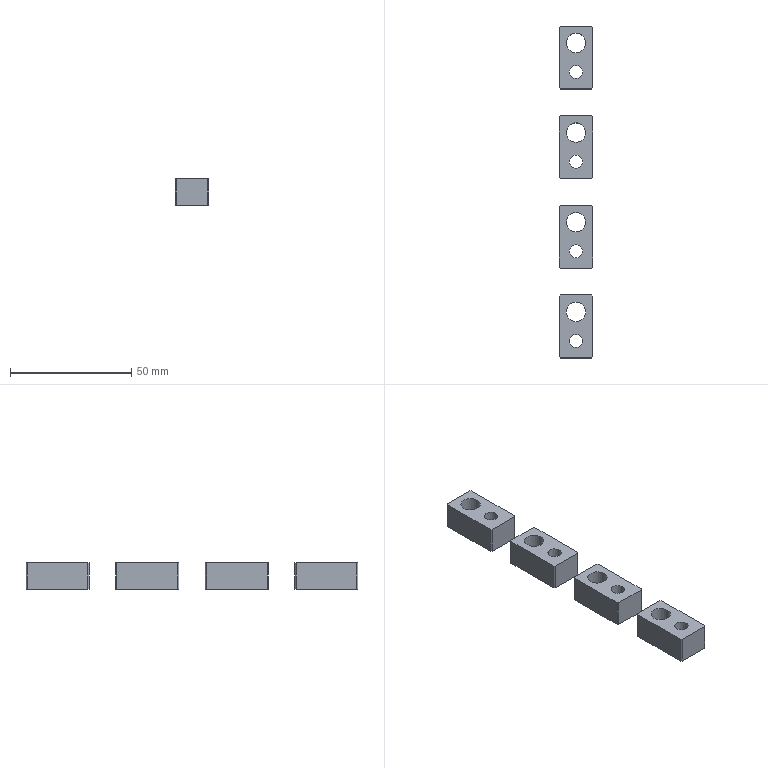Part | 4 solids | 56 faces | box 14 x 137 x 11 mm | volume 11860 mm3 | plane 44 | cylinder 12 | commonest cylinder face diameters 5.5 x4 8 x4 9 x4
STEP:
#1=CARTESIAN_POINT('',(-323.995,269.879,-17.));
#2=VERTEX_POINT('',#1);
#3=CARTESIAN_POINT('',(-321.245,269.879,-17.));
#4=DIRECTION('',(0.,0.,-1.));
#5=DIRECTION('',(-1.,0.,0.));
#6=AXIS2_PLACEMENT_3D('',#3,#4,#5);
#7=CIRCLE('',#6,2.75);
#8=EDGE_CURVE('',#2,#2,#7,.T.);
#9=ORIENTED_EDGE('',*,*,#8,.T.);
#10=EDGE_LOOP('',(#9));
#11=FACE_BOUND('',#10,.T.);
#12=CARTESIAN_POINT('',(-317.245,281.879,-17.));
#13=VERTEX_POINT('',#12);
#14=CARTESIAN_POINT('',(-321.245,281.879,-17.));
#15=DIRECTION('',(0.,0.,1.));
#16=DIRECTION('',(1.,0.,0.));
#17=AXIS2_PLACEMENT_3D('',#14,#15,#16);
#18=CIRCLE('',#17,4.);
#19=EDGE_CURVE('',#13,#13,#18,.T.);
#20=ORIENTED_EDGE('',*,*,#19,.F.);
#21=EDGE_LOOP('',(#20));
#22=FACE_BOUND('',#21,.T.);
#23=CARTESIAN_POINT('',(-328.245,288.379,-17.));
#24=VERTEX_POINT('',#23);
#25=CARTESIAN_POINT('',(-327.745,288.879,-17.));
#26=VERTEX_POINT('',#25);
#27=CARTESIAN_POINT('',(-333.995,282.629,-17.));
#28=DIRECTION('',(0.7071,0.7071,0.));
#29=VECTOR('',#28,1000.);
#30=LINE('',#27,#29);
#31=EDGE_CURVE('',#24,#26,#30,.T.);
#32=ORIENTED_EDGE('',*,*,#31,.F.);
#33=CARTESIAN_POINT('',(-328.245,263.379,-17.));
#34=VERTEX_POINT('',#33);
#35=CARTESIAN_POINT('',(-328.245,269.879,-17.));
#36=DIRECTION('',(0.,-1.,0.));
#37=VECTOR('',#36,1000.);
#38=LINE('',#35,#37);
#39=EDGE_CURVE('',#24,#34,#38,.T.);
#40=ORIENTED_EDGE('',*,*,#39,.T.);
#41=CARTESIAN_POINT('',(-327.745,262.879,-17.));
#42=VERTEX_POINT('',#41);
#43=CARTESIAN_POINT('',(-327.995,263.129,-17.));
#44=DIRECTION('',(-0.7071,0.7071,0.));
#45=VECTOR('',#44,1000.);
#46=LINE('',#43,#45);
#47=EDGE_CURVE('',#42,#34,#46,.T.);
#48=ORIENTED_EDGE('',*,*,#47,.F.);
#49=CARTESIAN_POINT('',(-314.745,262.879,-17.));
#50=VERTEX_POINT('',#49);
#51=CARTESIAN_POINT('',(-321.245,262.879,-17.));
#52=DIRECTION('',(1.,0.,0.));
#53=VECTOR('',#52,1000.);
#54=LINE('',#51,#53);
#55=EDGE_CURVE('',#42,#50,#54,.T.);
#56=ORIENTED_EDGE('',*,*,#55,.T.);
#57=CARTESIAN_POINT('',(-314.245,263.379,-17.));
#58=VERTEX_POINT('',#57);
#59=CARTESIAN_POINT('',(-314.495,263.129,-17.));
#60=DIRECTION('',(-0.7071,-0.7071,0.));
#61=VECTOR('',#60,1000.);
#62=LINE('',#59,#61);
#63=EDGE_CURVE('',#58,#50,#62,.T.);
#64=ORIENTED_EDGE('',*,*,#63,.F.);
#65=CARTESIAN_POINT('',(-314.245,288.379,-17.));
#66=VERTEX_POINT('',#65);
#67=CARTESIAN_POINT('',(-314.245,269.879,-17.));
#68=DIRECTION('',(0.,1.,0.));
#69=VECTOR('',#68,1000.);
#70=LINE('',#67,#69);
#71=EDGE_CURVE('',#58,#66,#70,.T.);
#72=ORIENTED_EDGE('',*,*,#71,.T.);
#73=CARTESIAN_POINT('',(-314.745,288.879,-17.));
#74=VERTEX_POINT('',#73);
#75=CARTESIAN_POINT('',(-308.495,282.629,-17.));
#76=DIRECTION('',(0.7071,-0.7071,0.));
#77=VECTOR('',#76,1000.);
#78=LINE('',#75,#77);
#79=EDGE_CURVE('',#74,#66,#78,.T.);
#80=ORIENTED_EDGE('',*,*,#79,.F.);
#81=CARTESIAN_POINT('',(-321.245,288.879,-17.));
#82=DIRECTION('',(-1.,0.,0.));
#83=VECTOR('',#82,1000.);
#84=LINE('',#81,#83);
#85=EDGE_CURVE('',#74,#26,#84,.T.);
#86=ORIENTED_EDGE('',*,*,#85,.T.);
#87=EDGE_LOOP('',(#32,#40,#48,#56,#64,#72,#80,#86));
#88=FACE_BOUND('',#87,.T.);
#89=CARTESIAN_POINT('',(-321.245,269.879,-17.));
#90=DIRECTION('',(0.,0.,1.));
#91=DIRECTION('',(-1.,0.,0.));
#92=AXIS2_PLACEMENT_3D('',#89,#90,#91);
#93=PLANE('',#92);
#94=ADVANCED_FACE('',(#11,#22,#88),#93,.T.);
#95=ORIENTED_EDGE('',*,*,#55,.F.);
#96=CARTESIAN_POINT('',(-327.745,262.879,-28.));
#97=VERTEX_POINT('',#96);
#98=CARTESIAN_POINT('',(-327.745,262.879,-16.));
#99=DIRECTION('',(0.,0.,-1.));
#100=VECTOR('',#99,1000.);
#101=LINE('',#98,#100);
#102=EDGE_CURVE('',#42,#97,#101,.T.);
#103=ORIENTED_EDGE('',*,*,#102,.T.);
#104=CARTESIAN_POINT('',(-314.745,262.879,-28.));
#105=VERTEX_POINT('',#104);
#106=CARTESIAN_POINT('',(-321.245,262.879,-28.));
#107=DIRECTION('',(-1.,0.,0.));
#108=VECTOR('',#107,1000.);
#109=LINE('',#106,#108);
#110=EDGE_CURVE('',#105,#97,#109,.T.);
#111=ORIENTED_EDGE('',*,*,#110,.F.);
#112=CARTESIAN_POINT('',(-314.745,262.879,-16.));
#113=DIRECTION('',(0.,0.,1.));
#114=VECTOR('',#113,1000.);
#115=LINE('',#112,#114);
#116=EDGE_CURVE('',#105,#50,#115,.T.);
#117=ORIENTED_EDGE('',*,*,#116,.T.);
#118=EDGE_LOOP('',(#95,#103,#111,#117));
#119=FACE_BOUND('',#118,.T.);
#120=CARTESIAN_POINT('',(-321.245,262.879,-16.));
#121=DIRECTION('',(0.,-1.,0.));
#122=DIRECTION('',(0.,0.,1.));
#123=AXIS2_PLACEMENT_3D('',#120,#121,#122);
#124=PLANE('',#123);
#125=ADVANCED_FACE('',(#119),#124,.T.);
#126=CARTESIAN_POINT('',(-314.245,263.379,-28.));
#127=VERTEX_POINT('',#126);
#128=CARTESIAN_POINT('',(-314.245,263.379,-16.));
#129=DIRECTION('',(0.,0.,-1.));
#130=VECTOR('',#129,1000.);
#131=LINE('',#128,#130);
#132=EDGE_CURVE('',#58,#127,#131,.T.);
#133=ORIENTED_EDGE('',*,*,#132,.F.);
#134=ORIENTED_EDGE('',*,*,#63,.T.);
#135=ORIENTED_EDGE('',*,*,#116,.F.);
#136=CARTESIAN_POINT('',(-314.495,263.129,-28.));
#137=DIRECTION('',(0.7071,0.7071,0.));
#138=VECTOR('',#137,1000.);
#139=LINE('',#136,#138);
#140=EDGE_CURVE('',#105,#127,#139,.T.);
#141=ORIENTED_EDGE('',*,*,#140,.T.);
#142=EDGE_LOOP('',(#133,#134,#135,#141));
#143=FACE_BOUND('',#142,.T.);
#144=CARTESIAN_POINT('',(-314.745,262.879,-16.));
#145=DIRECTION('',(-0.7071,0.7071,0.));
#146=DIRECTION('',(0.,0.,1.));
#147=AXIS2_PLACEMENT_3D('',#144,#145,#146);
#148=PLANE('',#147);
#149=ADVANCED_FACE('',(#143),#148,.F.);
#150=ORIENTED_EDGE('',*,*,#71,.F.);
#151=ORIENTED_EDGE('',*,*,#132,.T.);
#152=CARTESIAN_POINT('',(-314.245,288.379,-28.));
#153=VERTEX_POINT('',#152);
#154=CARTESIAN_POINT('',(-314.245,269.879,-28.));
#155=DIRECTION('',(0.,-1.,0.));
#156=VECTOR('',#155,1000.);
#157=LINE('',#154,#156);
#158=EDGE_CURVE('',#153,#127,#157,.T.);
#159=ORIENTED_EDGE('',*,*,#158,.F.);
#160=CARTESIAN_POINT('',(-314.245,288.379,-16.));
#161=DIRECTION('',(0.,0.,1.));
#162=VECTOR('',#161,1000.);
#163=LINE('',#160,#162);
#164=EDGE_CURVE('',#153,#66,#163,.T.);
#165=ORIENTED_EDGE('',*,*,#164,.T.);
#166=EDGE_LOOP('',(#150,#151,#159,#165));
#167=FACE_BOUND('',#166,.T.);
#168=CARTESIAN_POINT('',(-314.245,269.879,-16.));
#169=DIRECTION('',(1.,0.,0.));
#170=DIRECTION('',(0.,0.,1.));
#171=AXIS2_PLACEMENT_3D('',#168,#169,#170);
#172=PLANE('',#171);
#173=ADVANCED_FACE('',(#167),#172,.T.);
#174=CARTESIAN_POINT('',(-314.745,288.879,-28.));
#175=VERTEX_POINT('',#174);
#176=CARTESIAN_POINT('',(-314.745,288.879,-16.));
#177=DIRECTION('',(0.,0.,-1.));
#178=VECTOR('',#177,1000.);
#179=LINE('',#176,#178);
#180=EDGE_CURVE('',#74,#175,#179,.T.);
#181=ORIENTED_EDGE('',*,*,#180,.F.);
#182=ORIENTED_EDGE('',*,*,#79,.T.);
#183=ORIENTED_EDGE('',*,*,#164,.F.);
#184=CARTESIAN_POINT('',(-308.495,282.629,-28.));
#185=DIRECTION('',(-0.7071,0.7071,0.));
#186=VECTOR('',#185,1000.);
#187=LINE('',#184,#186);
#188=EDGE_CURVE('',#153,#175,#187,.T.);
#189=ORIENTED_EDGE('',*,*,#188,.T.);
#190=EDGE_LOOP('',(#181,#182,#183,#189));
#191=FACE_BOUND('',#190,.T.);
#192=CARTESIAN_POINT('',(-314.245,288.379,-16.));
#193=DIRECTION('',(-0.7071,-0.7071,0.));
#194=DIRECTION('',(0.,0.,1.));
#195=AXIS2_PLACEMENT_3D('',#192,#193,#194);
#196=PLANE('',#195);
#197=ADVANCED_FACE('',(#191),#196,.F.);
#198=ORIENTED_EDGE('',*,*,#85,.F.);
#199=ORIENTED_EDGE('',*,*,#180,.T.);
#200=CARTESIAN_POINT('',(-327.745,288.879,-28.));
#201=VERTEX_POINT('',#200);
#202=CARTESIAN_POINT('',(-321.245,288.879,-28.));
#203=DIRECTION('',(1.,0.,0.));
#204=VECTOR('',#203,1000.);
#205=LINE('',#202,#204);
#206=EDGE_CURVE('',#201,#175,#205,.T.);
#207=ORIENTED_EDGE('',*,*,#206,.F.);
#208=CARTESIAN_POINT('',(-327.745,288.879,-16.));
#209=DIRECTION('',(0.,0.,1.));
#210=VECTOR('',#209,1000.);
#211=LINE('',#208,#210);
#212=EDGE_CURVE('',#201,#26,#211,.T.);
#213=ORIENTED_EDGE('',*,*,#212,.T.);
#214=EDGE_LOOP('',(#198,#199,#207,#213));
#215=FACE_BOUND('',#214,.T.);
#216=CARTESIAN_POINT('',(-321.245,288.879,-16.));
#217=DIRECTION('',(0.,1.,0.));
#218=DIRECTION('',(0.,0.,-1.));
#219=AXIS2_PLACEMENT_3D('',#216,#217,#218);
#220=PLANE('',#219);
#221=ADVANCED_FACE('',(#215),#220,.T.);
#222=CARTESIAN_POINT('',(-328.245,288.379,-28.));
#223=VERTEX_POINT('',#222);
#224=CARTESIAN_POINT('',(-328.245,288.379,-16.));
#225=DIRECTION('',(0.,0.,-1.));
#226=VECTOR('',#225,1000.);
#227=LINE('',#224,#226);
#228=EDGE_CURVE('',#24,#223,#227,.T.);
#229=ORIENTED_EDGE('',*,*,#228,.F.);
#230=ORIENTED_EDGE('',*,*,#31,.T.);
#231=ORIENTED_EDGE('',*,*,#212,.F.);
#232=CARTESIAN_POINT('',(-333.995,282.629,-28.));
#233=DIRECTION('',(-0.7071,-0.7071,0.));
#234=VECTOR('',#233,1000.);
#235=LINE('',#232,#234);
#236=EDGE_CURVE('',#201,#223,#235,.T.);
#237=ORIENTED_EDGE('',*,*,#236,.T.);
#238=EDGE_LOOP('',(#229,#230,#231,#237));
#239=FACE_BOUND('',#238,.T.);
#240=CARTESIAN_POINT('',(-327.745,288.879,-16.));
#241=DIRECTION('',(0.7071,-0.7071,0.));
#242=DIRECTION('',(0.,0.,1.));
#243=AXIS2_PLACEMENT_3D('',#240,#241,#242);
#244=PLANE('',#243);
#245=ADVANCED_FACE('',(#239),#244,.F.);
#246=ORIENTED_EDGE('',*,*,#39,.F.);
#247=ORIENTED_EDGE('',*,*,#228,.T.);
#248=CARTESIAN_POINT('',(-328.245,263.379,-28.));
#249=VERTEX_POINT('',#248);
#250=CARTESIAN_POINT('',(-328.245,269.879,-28.));
#251=DIRECTION('',(0.,1.,0.));
#252=VECTOR('',#251,1000.);
#253=LINE('',#250,#252);
#254=EDGE_CURVE('',#249,#223,#253,.T.);
#255=ORIENTED_EDGE('',*,*,#254,.F.);
#256=CARTESIAN_POINT('',(-328.245,263.379,-16.));
#257=DIRECTION('',(0.,0.,1.));
#258=VECTOR('',#257,1000.);
#259=LINE('',#256,#258);
#260=EDGE_CURVE('',#249,#34,#259,.T.);
#261=ORIENTED_EDGE('',*,*,#260,.T.);
#262=EDGE_LOOP('',(#246,#247,#255,#261));
#263=FACE_BOUND('',#262,.T.);
#264=CARTESIAN_POINT('',(-328.245,269.879,-16.));
#265=DIRECTION('',(-1.,0.,0.));
#266=DIRECTION('',(0.,0.,-1.));
#267=AXIS2_PLACEMENT_3D('',#264,#265,#266);
#268=PLANE('',#267);
#269=ADVANCED_FACE('',(#263),#268,.T.);
#270=ORIENTED_EDGE('',*,*,#102,.F.);
#271=ORIENTED_EDGE('',*,*,#47,.T.);
#272=ORIENTED_EDGE('',*,*,#260,.F.);
#273=CARTESIAN_POINT('',(-327.995,263.129,-28.));
#274=DIRECTION('',(0.7071,-0.7071,0.));
#275=VECTOR('',#274,1000.);
#276=LINE('',#273,#275);
#277=EDGE_CURVE('',#249,#97,#276,.T.);
#278=ORIENTED_EDGE('',*,*,#277,.T.);
#279=EDGE_LOOP('',(#270,#271,#272,#278));
#280=FACE_BOUND('',#279,.T.);
#281=CARTESIAN_POINT('',(-328.245,263.379,-16.));
#282=DIRECTION('',(0.7071,0.7071,0.));
#283=DIRECTION('',(0.,0.,1.));
#284=AXIS2_PLACEMENT_3D('',#281,#282,#283);
#285=PLANE('',#284);
#286=ADVANCED_FACE('',(#280),#285,.F.);
#287=CARTESIAN_POINT('',(-325.745,269.879,-22.5));
#288=VERTEX_POINT('',#287);
#289=CARTESIAN_POINT('',(-321.245,269.879,-22.5));
#290=DIRECTION('',(0.,0.,1.));
#291=DIRECTION('',(-1.,0.,0.));
#292=AXIS2_PLACEMENT_3D('',#289,#290,#291);
#293=CIRCLE('',#292,4.5);
#294=EDGE_CURVE('',#288,#288,#293,.T.);
#295=ORIENTED_EDGE('',*,*,#294,.T.);
#296=EDGE_LOOP('',(#295));
#297=FACE_BOUND('',#296,.T.);
#298=CARTESIAN_POINT('',(-325.745,269.879,-28.));
#299=VERTEX_POINT('',#298);
#300=CARTESIAN_POINT('',(-321.245,269.879,-28.));
#301=DIRECTION('',(0.,0.,-1.));
#302=DIRECTION('',(-1.,0.,0.));
#303=AXIS2_PLACEMENT_3D('',#300,#301,#302);
#304=CIRCLE('',#303,4.5);
#305=EDGE_CURVE('',#299,#299,#304,.T.);
#306=ORIENTED_EDGE('',*,*,#305,.T.);
#307=EDGE_LOOP('',(#306));
#308=FACE_BOUND('',#307,.T.);
#309=CARTESIAN_POINT('',(-321.245,269.879,-28.));
#310=DIRECTION('',(0.,0.,1.));
#311=DIRECTION('',(-1.,0.,0.));
#312=AXIS2_PLACEMENT_3D('',#309,#310,#311);
#313=CYLINDRICAL_SURFACE('',#312,4.5);
#314=ADVANCED_FACE('',(#297,#308),#313,.F.);
#315=CARTESIAN_POINT('',(-323.995,269.879,-22.5));
#316=VERTEX_POINT('',#315);
#317=CARTESIAN_POINT('',(-321.245,269.879,-22.5));
#318=DIRECTION('',(0.,0.,-1.));
#319=DIRECTION('',(-1.,0.,0.));
#320=AXIS2_PLACEMENT_3D('',#317,#318,#319);
#321=CIRCLE('',#320,2.75);
#322=EDGE_CURVE('',#316,#316,#321,.T.);
#323=ORIENTED_EDGE('',*,*,#322,.F.);
#324=EDGE_LOOP('',(#323));
#325=FACE_BOUND('',#324,.T.);
#326=ORIENTED_EDGE('',*,*,#294,.F.);
#327=EDGE_LOOP('',(#326));
#328=FACE_BOUND('',#327,.T.);
#329=CARTESIAN_POINT('',(-321.245,269.879,-22.5));
#330=DIRECTION('',(0.,0.,1.));
#331=DIRECTION('',(-1.,0.,0.));
#332=AXIS2_PLACEMENT_3D('',#329,#330,#331);
#333=PLANE('',#332);
#334=ADVANCED_FACE('',(#325,#328),#333,.F.);
#335=ORIENTED_EDGE('',*,*,#8,.F.);
#336=EDGE_LOOP('',(#335));
#337=FACE_BOUND('',#336,.T.);
#338=ORIENTED_EDGE('',*,*,#322,.T.);
#339=EDGE_LOOP('',(#338));
#340=FACE_BOUND('',#339,.T.);
#341=CARTESIAN_POINT('',(-321.245,269.879,-17.));
#342=DIRECTION('',(0.,0.,-1.));
#343=DIRECTION('',(-1.,0.,0.));
#344=AXIS2_PLACEMENT_3D('',#341,#342,#343);
#345=CYLINDRICAL_SURFACE('',#344,2.75);
#346=ADVANCED_FACE('',(#337,#340),#345,.F.);
#347=CARTESIAN_POINT('',(-325.245,281.879,-28.));
#348=VERTEX_POINT('',#347);
#349=CARTESIAN_POINT('',(-321.245,281.879,-28.));
#350=DIRECTION('',(0.,0.,-1.));
#351=DIRECTION('',(-1.,0.,0.));
#352=AXIS2_PLACEMENT_3D('',#349,#350,#351);
#353=CIRCLE('',#352,4.);
#354=EDGE_CURVE('',#348,#348,#353,.T.);
#355=ORIENTED_EDGE('',*,*,#354,.T.);
#356=EDGE_LOOP('',(#355));
#357=FACE_BOUND('',#356,.T.);
#358=ORIENTED_EDGE('',*,*,#19,.T.);
#359=EDGE_LOOP('',(#358));
#360=FACE_BOUND('',#359,.T.);
#361=CARTESIAN_POINT('',(-321.245,281.879,-14.));
#362=DIRECTION('',(0.,0.,-1.));
#363=DIRECTION('',(-1.,0.,0.));
#364=AXIS2_PLACEMENT_3D('',#361,#362,#363);
#365=CYLINDRICAL_SURFACE('',#364,4.);
#366=ADVANCED_FACE('',(#357,#360),#365,.F.);
#367=ORIENTED_EDGE('',*,*,#305,.F.);
#368=EDGE_LOOP('',(#367));
#369=FACE_BOUND('',#368,.T.);
#370=ORIENTED_EDGE('',*,*,#140,.F.);
#371=ORIENTED_EDGE('',*,*,#110,.T.);
#372=ORIENTED_EDGE('',*,*,#277,.F.);
#373=ORIENTED_EDGE('',*,*,#254,.T.);
#374=ORIENTED_EDGE('',*,*,#236,.F.);
#375=ORIENTED_EDGE('',*,*,#206,.T.);
#376=ORIENTED_EDGE('',*,*,#188,.F.);
#377=ORIENTED_EDGE('',*,*,#158,.T.);
#378=EDGE_LOOP('',(#370,#371,#372,#373,#374,#375,#376,#377));
#379=FACE_BOUND('',#378,.T.);
#380=ORIENTED_EDGE('',*,*,#354,.F.);
#381=EDGE_LOOP('',(#380));
#382=FACE_BOUND('',#381,.T.);
#383=CARTESIAN_POINT('',(-321.245,269.879,-28.));
#384=DIRECTION('',(0.,0.,-1.));
#385=DIRECTION('',(1.,0.,0.));
#386=AXIS2_PLACEMENT_3D('',#383,#384,#385);
#387=PLANE('',#386);
#388=ADVANCED_FACE('',(#369,#379,#382),#387,.T.);
#389=CLOSED_SHELL('',(#94,#125,#149,#173,#197,#221,#245,#269,#286,#314,#334,#346,#366,#388));
#390=MANIFOLD_SOLID_BREP('',#389);
#391=CARTESIAN_POINT('',(-323.995,195.879,-17.));
#392=VERTEX_POINT('',#391);
#393=CARTESIAN_POINT('',(-321.245,195.879,-17.));
#394=DIRECTION('',(0.,0.,-1.));
#395=DIRECTION('',(-1.,0.,0.));
#396=AXIS2_PLACEMENT_3D('',#393,#394,#395);
#397=CIRCLE('',#396,2.75);
#398=EDGE_CURVE('',#392,#392,#397,.T.);
#399=ORIENTED_EDGE('',*,*,#398,.T.);
#400=EDGE_LOOP('',(#399));
#401=FACE_BOUND('',#400,.T.);
#402=CARTESIAN_POINT('',(-317.245,207.879,-17.));
#403=VERTEX_POINT('',#402);
#404=CARTESIAN_POINT('',(-321.245,207.879,-17.));
#405=DIRECTION('',(0.,0.,1.));
#406=DIRECTION('',(1.,0.,0.));
#407=AXIS2_PLACEMENT_3D('',#404,#405,#406);
#408=CIRCLE('',#407,4.);
#409=EDGE_CURVE('',#403,#403,#408,.T.);
#410=ORIENTED_EDGE('',*,*,#409,.F.);
#411=EDGE_LOOP('',(#410));
#412=FACE_BOUND('',#411,.T.);
#413=CARTESIAN_POINT('',(-328.245,214.379,-17.));
#414=VERTEX_POINT('',#413);
#415=CARTESIAN_POINT('',(-327.745,214.879,-17.));
#416=VERTEX_POINT('',#415);
#417=CARTESIAN_POINT('',(-333.995,208.629,-17.));
#418=DIRECTION('',(0.7071,0.7071,0.));
#419=VECTOR('',#418,1000.);
#420=LINE('',#417,#419);
#421=EDGE_CURVE('',#414,#416,#420,.T.);
#422=ORIENTED_EDGE('',*,*,#421,.F.);
#423=CARTESIAN_POINT('',(-328.245,189.379,-17.));
#424=VERTEX_POINT('',#423);
#425=CARTESIAN_POINT('',(-328.245,195.879,-17.));
#426=DIRECTION('',(0.,-1.,0.));
#427=VECTOR('',#426,1000.);
#428=LINE('',#425,#427);
#429=EDGE_CURVE('',#414,#424,#428,.T.);
#430=ORIENTED_EDGE('',*,*,#429,.T.);
#431=CARTESIAN_POINT('',(-327.745,188.879,-17.));
#432=VERTEX_POINT('',#431);
#433=CARTESIAN_POINT('',(-327.995,189.129,-17.));
#434=DIRECTION('',(-0.7071,0.7071,0.));
#435=VECTOR('',#434,1000.);
#436=LINE('',#433,#435);
#437=EDGE_CURVE('',#432,#424,#436,.T.);
#438=ORIENTED_EDGE('',*,*,#437,.F.);
#439=CARTESIAN_POINT('',(-314.745,188.879,-17.));
#440=VERTEX_POINT('',#439);
#441=CARTESIAN_POINT('',(-321.245,188.879,-17.));
#442=DIRECTION('',(1.,0.,0.));
#443=VECTOR('',#442,1000.);
#444=LINE('',#441,#443);
#445=EDGE_CURVE('',#432,#440,#444,.T.);
#446=ORIENTED_EDGE('',*,*,#445,.T.);
#447=CARTESIAN_POINT('',(-314.245,189.379,-17.));
#448=VERTEX_POINT('',#447);
#449=CARTESIAN_POINT('',(-314.495,189.129,-17.));
#450=DIRECTION('',(-0.7071,-0.7071,0.));
#451=VECTOR('',#450,1000.);
#452=LINE('',#449,#451);
#453=EDGE_CURVE('',#448,#440,#452,.T.);
#454=ORIENTED_EDGE('',*,*,#453,.F.);
#455=CARTESIAN_POINT('',(-314.245,214.379,-17.));
#456=VERTEX_POINT('',#455);
#457=CARTESIAN_POINT('',(-314.245,195.879,-17.));
#458=DIRECTION('',(0.,1.,0.));
#459=VECTOR('',#458,1000.);
#460=LINE('',#457,#459);
#461=EDGE_CURVE('',#448,#456,#460,.T.);
#462=ORIENTED_EDGE('',*,*,#461,.T.);
#463=CARTESIAN_POINT('',(-314.745,214.879,-17.));
#464=VERTEX_POINT('',#463);
#465=CARTESIAN_POINT('',(-308.495,208.629,-17.));
#466=DIRECTION('',(0.7071,-0.7071,0.));
#467=VECTOR('',#466,1000.);
#468=LINE('',#465,#467);
#469=EDGE_CURVE('',#464,#456,#468,.T.);
#470=ORIENTED_EDGE('',*,*,#469,.F.);
#471=CARTESIAN_POINT('',(-321.245,214.879,-17.));
#472=DIRECTION('',(-1.,0.,0.));
#473=VECTOR('',#472,1000.);
#474=LINE('',#471,#473);
#475=EDGE_CURVE('',#464,#416,#474,.T.);
#476=ORIENTED_EDGE('',*,*,#475,.T.);
#477=EDGE_LOOP('',(#422,#430,#438,#446,#454,#462,#470,#476));
#478=FACE_BOUND('',#477,.T.);
#479=CARTESIAN_POINT('',(-321.245,195.879,-17.));
#480=DIRECTION('',(0.,0.,1.));
#481=DIRECTION('',(-1.,0.,0.));
#482=AXIS2_PLACEMENT_3D('',#479,#480,#481);
#483=PLANE('',#482);
#484=ADVANCED_FACE('',(#401,#412,#478),#483,.T.);
#485=ORIENTED_EDGE('',*,*,#445,.F.);
#486=CARTESIAN_POINT('',(-327.745,188.879,-28.));
#487=VERTEX_POINT('',#486);
#488=CARTESIAN_POINT('',(-327.745,188.879,-16.));
#489=DIRECTION('',(0.,0.,-1.));
#490=VECTOR('',#489,1000.);
#491=LINE('',#488,#490);
#492=EDGE_CURVE('',#432,#487,#491,.T.);
#493=ORIENTED_EDGE('',*,*,#492,.T.);
#494=CARTESIAN_POINT('',(-314.745,188.879,-28.));
#495=VERTEX_POINT('',#494);
#496=CARTESIAN_POINT('',(-321.245,188.879,-28.));
#497=DIRECTION('',(-1.,0.,0.));
#498=VECTOR('',#497,1000.);
#499=LINE('',#496,#498);
#500=EDGE_CURVE('',#495,#487,#499,.T.);
#501=ORIENTED_EDGE('',*,*,#500,.F.);
#502=CARTESIAN_POINT('',(-314.745,188.879,-16.));
#503=DIRECTION('',(0.,0.,1.));
#504=VECTOR('',#503,1000.);
#505=LINE('',#502,#504);
#506=EDGE_CURVE('',#495,#440,#505,.T.);
#507=ORIENTED_EDGE('',*,*,#506,.T.);
#508=EDGE_LOOP('',(#485,#493,#501,#507));
#509=FACE_BOUND('',#508,.T.);
#510=CARTESIAN_POINT('',(-321.245,188.879,-16.));
#511=DIRECTION('',(0.,-1.,0.));
#512=DIRECTION('',(0.,0.,1.));
#513=AXIS2_PLACEMENT_3D('',#510,#511,#512);
#514=PLANE('',#513);
#515=ADVANCED_FACE('',(#509),#514,.T.);
#516=CARTESIAN_POINT('',(-314.245,189.379,-28.));
#517=VERTEX_POINT('',#516);
#518=CARTESIAN_POINT('',(-314.245,189.379,-16.));
#519=DIRECTION('',(0.,0.,-1.));
#520=VECTOR('',#519,1000.);
#521=LINE('',#518,#520);
#522=EDGE_CURVE('',#448,#517,#521,.T.);
#523=ORIENTED_EDGE('',*,*,#522,.F.);
#524=ORIENTED_EDGE('',*,*,#453,.T.);
#525=ORIENTED_EDGE('',*,*,#506,.F.);
#526=CARTESIAN_POINT('',(-314.495,189.129,-28.));
#527=DIRECTION('',(0.7071,0.7071,0.));
#528=VECTOR('',#527,1000.);
#529=LINE('',#526,#528);
#530=EDGE_CURVE('',#495,#517,#529,.T.);
#531=ORIENTED_EDGE('',*,*,#530,.T.);
#532=EDGE_LOOP('',(#523,#524,#525,#531));
#533=FACE_BOUND('',#532,.T.);
#534=CARTESIAN_POINT('',(-314.745,188.879,-16.));
#535=DIRECTION('',(-0.7071,0.7071,0.));
#536=DIRECTION('',(0.,0.,1.));
#537=AXIS2_PLACEMENT_3D('',#534,#535,#536);
#538=PLANE('',#537);
#539=ADVANCED_FACE('',(#533),#538,.F.);
#540=ORIENTED_EDGE('',*,*,#461,.F.);
#541=ORIENTED_EDGE('',*,*,#522,.T.);
#542=CARTESIAN_POINT('',(-314.245,214.379,-28.));
#543=VERTEX_POINT('',#542);
#544=CARTESIAN_POINT('',(-314.245,195.879,-28.));
#545=DIRECTION('',(0.,-1.,0.));
#546=VECTOR('',#545,1000.);
#547=LINE('',#544,#546);
#548=EDGE_CURVE('',#543,#517,#547,.T.);
#549=ORIENTED_EDGE('',*,*,#548,.F.);
#550=CARTESIAN_POINT('',(-314.245,214.379,-16.));
#551=DIRECTION('',(0.,0.,1.));
#552=VECTOR('',#551,1000.);
#553=LINE('',#550,#552);
#554=EDGE_CURVE('',#543,#456,#553,.T.);
#555=ORIENTED_EDGE('',*,*,#554,.T.);
#556=EDGE_LOOP('',(#540,#541,#549,#555));
#557=FACE_BOUND('',#556,.T.);
#558=CARTESIAN_POINT('',(-314.245,195.879,-16.));
#559=DIRECTION('',(1.,0.,0.));
#560=DIRECTION('',(0.,0.,1.));
#561=AXIS2_PLACEMENT_3D('',#558,#559,#560);
#562=PLANE('',#561);
#563=ADVANCED_FACE('',(#557),#562,.T.);
#564=CARTESIAN_POINT('',(-314.745,214.879,-28.));
#565=VERTEX_POINT('',#564);
#566=CARTESIAN_POINT('',(-314.745,214.879,-16.));
#567=DIRECTION('',(0.,0.,-1.));
#568=VECTOR('',#567,1000.);
#569=LINE('',#566,#568);
#570=EDGE_CURVE('',#464,#565,#569,.T.);
#571=ORIENTED_EDGE('',*,*,#570,.F.);
#572=ORIENTED_EDGE('',*,*,#469,.T.);
#573=ORIENTED_EDGE('',*,*,#554,.F.);
#574=CARTESIAN_POINT('',(-308.495,208.629,-28.));
#575=DIRECTION('',(-0.7071,0.7071,0.));
#576=VECTOR('',#575,1000.);
#577=LINE('',#574,#576);
#578=EDGE_CURVE('',#543,#565,#577,.T.);
#579=ORIENTED_EDGE('',*,*,#578,.T.);
#580=EDGE_LOOP('',(#571,#572,#573,#579));
#581=FACE_BOUND('',#580,.T.);
#582=CARTESIAN_POINT('',(-314.245,214.379,-16.));
#583=DIRECTION('',(-0.7071,-0.7071,0.));
#584=DIRECTION('',(0.,0.,1.));
#585=AXIS2_PLACEMENT_3D('',#582,#583,#584);
#586=PLANE('',#585);
#587=ADVANCED_FACE('',(#581),#586,.F.);
#588=ORIENTED_EDGE('',*,*,#475,.F.);
#589=ORIENTED_EDGE('',*,*,#570,.T.);
#590=CARTESIAN_POINT('',(-327.745,214.879,-28.));
#591=VERTEX_POINT('',#590);
#592=CARTESIAN_POINT('',(-321.245,214.879,-28.));
#593=DIRECTION('',(1.,0.,0.));
#594=VECTOR('',#593,1000.);
#595=LINE('',#592,#594);
#596=EDGE_CURVE('',#591,#565,#595,.T.);
#597=ORIENTED_EDGE('',*,*,#596,.F.);
#598=CARTESIAN_POINT('',(-327.745,214.879,-16.));
#599=DIRECTION('',(0.,0.,1.));
#600=VECTOR('',#599,1000.);
#601=LINE('',#598,#600);
#602=EDGE_CURVE('',#591,#416,#601,.T.);
#603=ORIENTED_EDGE('',*,*,#602,.T.);
#604=EDGE_LOOP('',(#588,#589,#597,#603));
#605=FACE_BOUND('',#604,.T.);
#606=CARTESIAN_POINT('',(-321.245,214.879,-16.));
#607=DIRECTION('',(0.,1.,0.));
#608=DIRECTION('',(0.,0.,-1.));
#609=AXIS2_PLACEMENT_3D('',#606,#607,#608);
#610=PLANE('',#609);
#611=ADVANCED_FACE('',(#605),#610,.T.);
#612=CARTESIAN_POINT('',(-328.245,214.379,-28.));
#613=VERTEX_POINT('',#612);
#614=CARTESIAN_POINT('',(-328.245,214.379,-16.));
#615=DIRECTION('',(0.,0.,-1.));
#616=VECTOR('',#615,1000.);
#617=LINE('',#614,#616);
#618=EDGE_CURVE('',#414,#613,#617,.T.);
#619=ORIENTED_EDGE('',*,*,#618,.F.);
#620=ORIENTED_EDGE('',*,*,#421,.T.);
#621=ORIENTED_EDGE('',*,*,#602,.F.);
#622=CARTESIAN_POINT('',(-333.995,208.629,-28.));
#623=DIRECTION('',(-0.7071,-0.7071,0.));
#624=VECTOR('',#623,1000.);
#625=LINE('',#622,#624);
#626=EDGE_CURVE('',#591,#613,#625,.T.);
#627=ORIENTED_EDGE('',*,*,#626,.T.);
#628=EDGE_LOOP('',(#619,#620,#621,#627));
#629=FACE_BOUND('',#628,.T.);
#630=CARTESIAN_POINT('',(-327.745,214.879,-16.));
#631=DIRECTION('',(0.7071,-0.7071,0.));
#632=DIRECTION('',(0.,0.,1.));
#633=AXIS2_PLACEMENT_3D('',#630,#631,#632);
#634=PLANE('',#633);
#635=ADVANCED_FACE('',(#629),#634,.F.);
#636=ORIENTED_EDGE('',*,*,#429,.F.);
#637=ORIENTED_EDGE('',*,*,#618,.T.);
#638=CARTESIAN_POINT('',(-328.245,189.379,-28.));
#639=VERTEX_POINT('',#638);
#640=CARTESIAN_POINT('',(-328.245,195.879,-28.));
#641=DIRECTION('',(0.,1.,0.));
#642=VECTOR('',#641,1000.);
#643=LINE('',#640,#642);
#644=EDGE_CURVE('',#639,#613,#643,.T.);
#645=ORIENTED_EDGE('',*,*,#644,.F.);
#646=CARTESIAN_POINT('',(-328.245,189.379,-16.));
#647=DIRECTION('',(0.,0.,1.));
#648=VECTOR('',#647,1000.);
#649=LINE('',#646,#648);
#650=EDGE_CURVE('',#639,#424,#649,.T.);
#651=ORIENTED_EDGE('',*,*,#650,.T.);
#652=EDGE_LOOP('',(#636,#637,#645,#651));
#653=FACE_BOUND('',#652,.T.);
#654=CARTESIAN_POINT('',(-328.245,195.879,-16.));
#655=DIRECTION('',(-1.,0.,0.));
#656=DIRECTION('',(0.,0.,-1.));
#657=AXIS2_PLACEMENT_3D('',#654,#655,#656);
#658=PLANE('',#657);
#659=ADVANCED_FACE('',(#653),#658,.T.);
#660=ORIENTED_EDGE('',*,*,#492,.F.);
#661=ORIENTED_EDGE('',*,*,#437,.T.);
#662=ORIENTED_EDGE('',*,*,#650,.F.);
#663=CARTESIAN_POINT('',(-327.995,189.129,-28.));
#664=DIRECTION('',(0.7071,-0.7071,0.));
#665=VECTOR('',#664,1000.);
#666=LINE('',#663,#665);
#667=EDGE_CURVE('',#639,#487,#666,.T.);
#668=ORIENTED_EDGE('',*,*,#667,.T.);
#669=EDGE_LOOP('',(#660,#661,#662,#668));
#670=FACE_BOUND('',#669,.T.);
#671=CARTESIAN_POINT('',(-328.245,189.379,-16.));
#672=DIRECTION('',(0.7071,0.7071,0.));
#673=DIRECTION('',(0.,0.,1.));
#674=AXIS2_PLACEMENT_3D('',#671,#672,#673);
#675=PLANE('',#674);
#676=ADVANCED_FACE('',(#670),#675,.F.);
#677=CARTESIAN_POINT('',(-325.745,195.879,-22.5));
#678=VERTEX_POINT('',#677);
#679=CARTESIAN_POINT('',(-321.245,195.879,-22.5));
#680=DIRECTION('',(0.,0.,1.));
#681=DIRECTION('',(-1.,0.,0.));
#682=AXIS2_PLACEMENT_3D('',#679,#680,#681);
#683=CIRCLE('',#682,4.5);
#684=EDGE_CURVE('',#678,#678,#683,.T.);
#685=ORIENTED_EDGE('',*,*,#684,.T.);
#686=EDGE_LOOP('',(#685));
#687=FACE_BOUND('',#686,.T.);
#688=CARTESIAN_POINT('',(-325.745,195.879,-28.));
#689=VERTEX_POINT('',#688);
#690=CARTESIAN_POINT('',(-321.245,195.879,-28.));
#691=DIRECTION('',(0.,0.,-1.));
#692=DIRECTION('',(-1.,0.,0.));
#693=AXIS2_PLACEMENT_3D('',#690,#691,#692);
#694=CIRCLE('',#693,4.5);
#695=EDGE_CURVE('',#689,#689,#694,.T.);
#696=ORIENTED_EDGE('',*,*,#695,.T.);
#697=EDGE_LOOP('',(#696));
#698=FACE_BOUND('',#697,.T.);
#699=CARTESIAN_POINT('',(-321.245,195.879,-28.));
#700=DIRECTION('',(0.,0.,1.));
#701=DIRECTION('',(-1.,0.,0.));
#702=AXIS2_PLACEMENT_3D('',#699,#700,#701);
#703=CYLINDRICAL_SURFACE('',#702,4.5);
#704=ADVANCED_FACE('',(#687,#698),#703,.F.);
#705=CARTESIAN_POINT('',(-323.995,195.879,-22.5));
#706=VERTEX_POINT('',#705);
#707=CARTESIAN_POINT('',(-321.245,195.879,-22.5));
#708=DIRECTION('',(0.,0.,-1.));
#709=DIRECTION('',(-1.,0.,0.));
#710=AXIS2_PLACEMENT_3D('',#707,#708,#709);
#711=CIRCLE('',#710,2.75);
#712=EDGE_CURVE('',#706,#706,#711,.T.);
#713=ORIENTED_EDGE('',*,*,#712,.F.);
#714=EDGE_LOOP('',(#713));
#715=FACE_BOUND('',#714,.T.);
#716=ORIENTED_EDGE('',*,*,#684,.F.);
#717=EDGE_LOOP('',(#716));
#718=FACE_BOUND('',#717,.T.);
#719=CARTESIAN_POINT('',(-321.245,195.879,-22.5));
#720=DIRECTION('',(0.,0.,1.));
#721=DIRECTION('',(-1.,0.,0.));
#722=AXIS2_PLACEMENT_3D('',#719,#720,#721);
#723=PLANE('',#722);
#724=ADVANCED_FACE('',(#715,#718),#723,.F.);
#725=ORIENTED_EDGE('',*,*,#398,.F.);
#726=EDGE_LOOP('',(#725));
#727=FACE_BOUND('',#726,.T.);
#728=ORIENTED_EDGE('',*,*,#712,.T.);
#729=EDGE_LOOP('',(#728));
#730=FACE_BOUND('',#729,.T.);
#731=CARTESIAN_POINT('',(-321.245,195.879,-17.));
#732=DIRECTION('',(0.,0.,-1.));
#733=DIRECTION('',(-1.,0.,0.));
#734=AXIS2_PLACEMENT_3D('',#731,#732,#733);
#735=CYLINDRICAL_SURFACE('',#734,2.75);
#736=ADVANCED_FACE('',(#727,#730),#735,.F.);
#737=CARTESIAN_POINT('',(-325.245,207.879,-28.));
#738=VERTEX_POINT('',#737);
#739=CARTESIAN_POINT('',(-321.245,207.879,-28.));
#740=DIRECTION('',(0.,0.,-1.));
#741=DIRECTION('',(-1.,0.,0.));
#742=AXIS2_PLACEMENT_3D('',#739,#740,#741);
#743=CIRCLE('',#742,4.);
#744=EDGE_CURVE('',#738,#738,#743,.T.);
#745=ORIENTED_EDGE('',*,*,#744,.T.);
#746=EDGE_LOOP('',(#745));
#747=FACE_BOUND('',#746,.T.);
#748=ORIENTED_EDGE('',*,*,#409,.T.);
#749=EDGE_LOOP('',(#748));
#750=FACE_BOUND('',#749,.T.);
#751=CARTESIAN_POINT('',(-321.245,207.879,-14.));
#752=DIRECTION('',(0.,0.,-1.));
#753=DIRECTION('',(-1.,0.,0.));
#754=AXIS2_PLACEMENT_3D('',#751,#752,#753);
#755=CYLINDRICAL_SURFACE('',#754,4.);
#756=ADVANCED_FACE('',(#747,#750),#755,.F.);
#757=ORIENTED_EDGE('',*,*,#695,.F.);
#758=EDGE_LOOP('',(#757));
#759=FACE_BOUND('',#758,.T.);
#760=ORIENTED_EDGE('',*,*,#530,.F.);
#761=ORIENTED_EDGE('',*,*,#500,.T.);
#762=ORIENTED_EDGE('',*,*,#667,.F.);
#763=ORIENTED_EDGE('',*,*,#644,.T.);
#764=ORIENTED_EDGE('',*,*,#626,.F.);
#765=ORIENTED_EDGE('',*,*,#596,.T.);
#766=ORIENTED_EDGE('',*,*,#578,.F.);
#767=ORIENTED_EDGE('',*,*,#548,.T.);
#768=EDGE_LOOP('',(#760,#761,#762,#763,#764,#765,#766,#767));
#769=FACE_BOUND('',#768,.T.);
#770=ORIENTED_EDGE('',*,*,#744,.F.);
#771=EDGE_LOOP('',(#770));
#772=FACE_BOUND('',#771,.T.);
#773=CARTESIAN_POINT('',(-321.245,195.879,-28.));
#774=DIRECTION('',(0.,0.,-1.));
#775=DIRECTION('',(1.,0.,0.));
#776=AXIS2_PLACEMENT_3D('',#773,#774,#775);
#777=PLANE('',#776);
#778=ADVANCED_FACE('',(#759,#769,#772),#777,.T.);
#779=CLOSED_SHELL('',(#484,#515,#539,#563,#587,#611,#635,#659,#676,#704,#724,#736,#756,#778));
#780=MANIFOLD_SOLID_BREP('',#779);
#781=CARTESIAN_POINT('',(-323.995,158.879,-17.));
#782=VERTEX_POINT('',#781);
#783=CARTESIAN_POINT('',(-321.245,158.879,-17.));
#784=DIRECTION('',(0.,0.,-1.));
#785=DIRECTION('',(-1.,0.,0.));
#786=AXIS2_PLACEMENT_3D('',#783,#784,#785);
#787=CIRCLE('',#786,2.75);
#788=EDGE_CURVE('',#782,#782,#787,.T.);
#789=ORIENTED_EDGE('',*,*,#788,.T.);
#790=EDGE_LOOP('',(#789));
#791=FACE_BOUND('',#790,.T.);
#792=CARTESIAN_POINT('',(-317.245,170.879,-17.));
#793=VERTEX_POINT('',#792);
#794=CARTESIAN_POINT('',(-321.245,170.879,-17.));
#795=DIRECTION('',(0.,0.,1.));
#796=DIRECTION('',(1.,0.,0.));
#797=AXIS2_PLACEMENT_3D('',#794,#795,#796);
#798=CIRCLE('',#797,4.);
#799=EDGE_CURVE('',#793,#793,#798,.T.);
#800=ORIENTED_EDGE('',*,*,#799,.F.);
#801=EDGE_LOOP('',(#800));
#802=FACE_BOUND('',#801,.T.);
#803=CARTESIAN_POINT('',(-328.245,177.379,-17.));
#804=VERTEX_POINT('',#803);
#805=CARTESIAN_POINT('',(-327.745,177.879,-17.));
#806=VERTEX_POINT('',#805);
#807=CARTESIAN_POINT('',(-333.995,171.629,-17.));
#808=DIRECTION('',(0.7071,0.7071,0.));
#809=VECTOR('',#808,1000.);
#810=LINE('',#807,#809);
#811=EDGE_CURVE('',#804,#806,#810,.T.);
#812=ORIENTED_EDGE('',*,*,#811,.F.);
#813=CARTESIAN_POINT('',(-328.245,152.379,-17.));
#814=VERTEX_POINT('',#813);
#815=CARTESIAN_POINT('',(-328.245,158.879,-17.));
#816=DIRECTION('',(0.,-1.,0.));
#817=VECTOR('',#816,1000.);
#818=LINE('',#815,#817);
#819=EDGE_CURVE('',#804,#814,#818,.T.);
#820=ORIENTED_EDGE('',*,*,#819,.T.);
#821=CARTESIAN_POINT('',(-327.745,151.879,-17.));
#822=VERTEX_POINT('',#821);
#823=CARTESIAN_POINT('',(-327.995,152.129,-17.));
#824=DIRECTION('',(-0.7071,0.7071,0.));
#825=VECTOR('',#824,1000.);
#826=LINE('',#823,#825);
#827=EDGE_CURVE('',#822,#814,#826,.T.);
#828=ORIENTED_EDGE('',*,*,#827,.F.);
#829=CARTESIAN_POINT('',(-314.745,151.879,-17.));
#830=VERTEX_POINT('',#829);
#831=CARTESIAN_POINT('',(-321.245,151.879,-17.));
#832=DIRECTION('',(1.,0.,0.));
#833=VECTOR('',#832,1000.);
#834=LINE('',#831,#833);
#835=EDGE_CURVE('',#822,#830,#834,.T.);
#836=ORIENTED_EDGE('',*,*,#835,.T.);
#837=CARTESIAN_POINT('',(-314.245,152.379,-17.));
#838=VERTEX_POINT('',#837);
#839=CARTESIAN_POINT('',(-314.495,152.129,-17.));
#840=DIRECTION('',(-0.7071,-0.7071,0.));
#841=VECTOR('',#840,1000.);
#842=LINE('',#839,#841);
#843=EDGE_CURVE('',#838,#830,#842,.T.);
#844=ORIENTED_EDGE('',*,*,#843,.F.);
#845=CARTESIAN_POINT('',(-314.245,177.379,-17.));
#846=VERTEX_POINT('',#845);
#847=CARTESIAN_POINT('',(-314.245,158.879,-17.));
#848=DIRECTION('',(0.,1.,0.));
#849=VECTOR('',#848,1000.);
#850=LINE('',#847,#849);
#851=EDGE_CURVE('',#838,#846,#850,.T.);
#852=ORIENTED_EDGE('',*,*,#851,.T.);
#853=CARTESIAN_POINT('',(-314.745,177.879,-17.));
#854=VERTEX_POINT('',#853);
#855=CARTESIAN_POINT('',(-308.495,171.629,-17.));
#856=DIRECTION('',(0.7071,-0.7071,0.));
#857=VECTOR('',#856,1000.);
#858=LINE('',#855,#857);
#859=EDGE_CURVE('',#854,#846,#858,.T.);
#860=ORIENTED_EDGE('',*,*,#859,.F.);
#861=CARTESIAN_POINT('',(-321.245,177.879,-17.));
#862=DIRECTION('',(-1.,0.,0.));
#863=VECTOR('',#862,1000.);
#864=LINE('',#861,#863);
#865=EDGE_CURVE('',#854,#806,#864,.T.);
#866=ORIENTED_EDGE('',*,*,#865,.T.);
#867=EDGE_LOOP('',(#812,#820,#828,#836,#844,#852,#860,#866));
#868=FACE_BOUND('',#867,.T.);
#869=CARTESIAN_POINT('',(-321.245,158.879,-17.));
#870=DIRECTION('',(0.,0.,1.));
#871=DIRECTION('',(-1.,0.,0.));
#872=AXIS2_PLACEMENT_3D('',#869,#870,#871);
#873=PLANE('',#872);
#874=ADVANCED_FACE('',(#791,#802,#868),#873,.T.);
#875=ORIENTED_EDGE('',*,*,#835,.F.);
#876=CARTESIAN_POINT('',(-327.745,151.879,-28.));
#877=VERTEX_POINT('',#876);
#878=CARTESIAN_POINT('',(-327.745,151.879,-16.));
#879=DIRECTION('',(0.,0.,-1.));
#880=VECTOR('',#879,1000.);
#881=LINE('',#878,#880);
#882=EDGE_CURVE('',#822,#877,#881,.T.);
#883=ORIENTED_EDGE('',*,*,#882,.T.);
#884=CARTESIAN_POINT('',(-314.745,151.879,-28.));
#885=VERTEX_POINT('',#884);
#886=CARTESIAN_POINT('',(-321.245,151.879,-28.));
#887=DIRECTION('',(-1.,0.,0.));
#888=VECTOR('',#887,1000.);
#889=LINE('',#886,#888);
#890=EDGE_CURVE('',#885,#877,#889,.T.);
#891=ORIENTED_EDGE('',*,*,#890,.F.);
#892=CARTESIAN_POINT('',(-314.745,151.879,-16.));
#893=DIRECTION('',(0.,0.,1.));
#894=VECTOR('',#893,1000.);
#895=LINE('',#892,#894);
#896=EDGE_CURVE('',#885,#830,#895,.T.);
#897=ORIENTED_EDGE('',*,*,#896,.T.);
#898=EDGE_LOOP('',(#875,#883,#891,#897));
#899=FACE_BOUND('',#898,.T.);
#900=CARTESIAN_POINT('',(-321.245,151.879,-16.));
#901=DIRECTION('',(0.,-1.,0.));
#902=DIRECTION('',(0.,0.,1.));
#903=AXIS2_PLACEMENT_3D('',#900,#901,#902);
#904=PLANE('',#903);
#905=ADVANCED_FACE('',(#899),#904,.T.);
#906=CARTESIAN_POINT('',(-314.245,152.379,-28.));
#907=VERTEX_POINT('',#906);
#908=CARTESIAN_POINT('',(-314.245,152.379,-16.));
#909=DIRECTION('',(0.,0.,-1.));
#910=VECTOR('',#909,1000.);
#911=LINE('',#908,#910);
#912=EDGE_CURVE('',#838,#907,#911,.T.);
#913=ORIENTED_EDGE('',*,*,#912,.F.);
#914=ORIENTED_EDGE('',*,*,#843,.T.);
#915=ORIENTED_EDGE('',*,*,#896,.F.);
#916=CARTESIAN_POINT('',(-314.495,152.129,-28.));
#917=DIRECTION('',(0.7071,0.7071,0.));
#918=VECTOR('',#917,1000.);
#919=LINE('',#916,#918);
#920=EDGE_CURVE('',#885,#907,#919,.T.);
#921=ORIENTED_EDGE('',*,*,#920,.T.);
#922=EDGE_LOOP('',(#913,#914,#915,#921));
#923=FACE_BOUND('',#922,.T.);
#924=CARTESIAN_POINT('',(-314.745,151.879,-16.));
#925=DIRECTION('',(-0.7071,0.7071,0.));
#926=DIRECTION('',(0.,0.,1.));
#927=AXIS2_PLACEMENT_3D('',#924,#925,#926);
#928=PLANE('',#927);
#929=ADVANCED_FACE('',(#923),#928,.F.);
#930=ORIENTED_EDGE('',*,*,#851,.F.);
#931=ORIENTED_EDGE('',*,*,#912,.T.);
#932=CARTESIAN_POINT('',(-314.245,177.379,-28.));
#933=VERTEX_POINT('',#932);
#934=CARTESIAN_POINT('',(-314.245,158.879,-28.));
#935=DIRECTION('',(0.,-1.,0.));
#936=VECTOR('',#935,1000.);
#937=LINE('',#934,#936);
#938=EDGE_CURVE('',#933,#907,#937,.T.);
#939=ORIENTED_EDGE('',*,*,#938,.F.);
#940=CARTESIAN_POINT('',(-314.245,177.379,-16.));
#941=DIRECTION('',(0.,0.,1.));
#942=VECTOR('',#941,1000.);
#943=LINE('',#940,#942);
#944=EDGE_CURVE('',#933,#846,#943,.T.);
#945=ORIENTED_EDGE('',*,*,#944,.T.);
#946=EDGE_LOOP('',(#930,#931,#939,#945));
#947=FACE_BOUND('',#946,.T.);
#948=CARTESIAN_POINT('',(-314.245,158.879,-16.));
#949=DIRECTION('',(1.,0.,0.));
#950=DIRECTION('',(0.,0.,1.));
#951=AXIS2_PLACEMENT_3D('',#948,#949,#950);
#952=PLANE('',#951);
#953=ADVANCED_FACE('',(#947),#952,.T.);
#954=CARTESIAN_POINT('',(-314.745,177.879,-28.));
#955=VERTEX_POINT('',#954);
#956=CARTESIAN_POINT('',(-314.745,177.879,-16.));
#957=DIRECTION('',(0.,0.,-1.));
#958=VECTOR('',#957,1000.);
#959=LINE('',#956,#958);
#960=EDGE_CURVE('',#854,#955,#959,.T.);
#961=ORIENTED_EDGE('',*,*,#960,.F.);
#962=ORIENTED_EDGE('',*,*,#859,.T.);
#963=ORIENTED_EDGE('',*,*,#944,.F.);
#964=CARTESIAN_POINT('',(-308.495,171.629,-28.));
#965=DIRECTION('',(-0.7071,0.7071,0.));
#966=VECTOR('',#965,1000.);
#967=LINE('',#964,#966);
#968=EDGE_CURVE('',#933,#955,#967,.T.);
#969=ORIENTED_EDGE('',*,*,#968,.T.);
#970=EDGE_LOOP('',(#961,#962,#963,#969));
#971=FACE_BOUND('',#970,.T.);
#972=CARTESIAN_POINT('',(-314.245,177.379,-16.));
#973=DIRECTION('',(-0.7071,-0.7071,0.));
#974=DIRECTION('',(0.,0.,1.));
#975=AXIS2_PLACEMENT_3D('',#972,#973,#974);
#976=PLANE('',#975);
#977=ADVANCED_FACE('',(#971),#976,.F.);
#978=ORIENTED_EDGE('',*,*,#865,.F.);
#979=ORIENTED_EDGE('',*,*,#960,.T.);
#980=CARTESIAN_POINT('',(-327.745,177.879,-28.));
#981=VERTEX_POINT('',#980);
#982=CARTESIAN_POINT('',(-321.245,177.879,-28.));
#983=DIRECTION('',(1.,0.,0.));
#984=VECTOR('',#983,1000.);
#985=LINE('',#982,#984);
#986=EDGE_CURVE('',#981,#955,#985,.T.);
#987=ORIENTED_EDGE('',*,*,#986,.F.);
#988=CARTESIAN_POINT('',(-327.745,177.879,-16.));
#989=DIRECTION('',(0.,0.,1.));
#990=VECTOR('',#989,1000.);
#991=LINE('',#988,#990);
#992=EDGE_CURVE('',#981,#806,#991,.T.);
#993=ORIENTED_EDGE('',*,*,#992,.T.);
#994=EDGE_LOOP('',(#978,#979,#987,#993));
#995=FACE_BOUND('',#994,.T.);
#996=CARTESIAN_POINT('',(-321.245,177.879,-16.));
#997=DIRECTION('',(0.,1.,0.));
#998=DIRECTION('',(0.,0.,-1.));
#999=AXIS2_PLACEMENT_3D('',#996,#997,#998);
#1000=PLANE('',#999);
#1001=ADVANCED_FACE('',(#995),#1000,.T.);
#1002=CARTESIAN_POINT('',(-328.245,177.379,-28.));
#1003=VERTEX_POINT('',#1002);
#1004=CARTESIAN_POINT('',(-328.245,177.379,-16.));
#1005=DIRECTION('',(0.,0.,-1.));
#1006=VECTOR('',#1005,1000.);
#1007=LINE('',#1004,#1006);
#1008=EDGE_CURVE('',#804,#1003,#1007,.T.);
#1009=ORIENTED_EDGE('',*,*,#1008,.F.);
#1010=ORIENTED_EDGE('',*,*,#811,.T.);
#1011=ORIENTED_EDGE('',*,*,#992,.F.);
#1012=CARTESIAN_POINT('',(-333.995,171.629,-28.));
#1013=DIRECTION('',(-0.7071,-0.7071,0.));
#1014=VECTOR('',#1013,1000.);
#1015=LINE('',#1012,#1014);
#1016=EDGE_CURVE('',#981,#1003,#1015,.T.);
#1017=ORIENTED_EDGE('',*,*,#1016,.T.);
#1018=EDGE_LOOP('',(#1009,#1010,#1011,#1017));
#1019=FACE_BOUND('',#1018,.T.);
#1020=CARTESIAN_POINT('',(-327.745,177.879,-16.));
#1021=DIRECTION('',(0.7071,-0.7071,0.));
#1022=DIRECTION('',(0.,0.,1.));
#1023=AXIS2_PLACEMENT_3D('',#1020,#1021,#1022);
#1024=PLANE('',#1023);
#1025=ADVANCED_FACE('',(#1019),#1024,.F.);
#1026=ORIENTED_EDGE('',*,*,#819,.F.);
#1027=ORIENTED_EDGE('',*,*,#1008,.T.);
#1028=CARTESIAN_POINT('',(-328.245,152.379,-28.));
#1029=VERTEX_POINT('',#1028);
#1030=CARTESIAN_POINT('',(-328.245,158.879,-28.));
#1031=DIRECTION('',(0.,1.,0.));
#1032=VECTOR('',#1031,1000.);
#1033=LINE('',#1030,#1032);
#1034=EDGE_CURVE('',#1029,#1003,#1033,.T.);
#1035=ORIENTED_EDGE('',*,*,#1034,.F.);
#1036=CARTESIAN_POINT('',(-328.245,152.379,-16.));
#1037=DIRECTION('',(0.,0.,1.));
#1038=VECTOR('',#1037,1000.);
#1039=LINE('',#1036,#1038);
#1040=EDGE_CURVE('',#1029,#814,#1039,.T.);
#1041=ORIENTED_EDGE('',*,*,#1040,.T.);
#1042=EDGE_LOOP('',(#1026,#1027,#1035,#1041));
#1043=FACE_BOUND('',#1042,.T.);
#1044=CARTESIAN_POINT('',(-328.245,158.879,-16.));
#1045=DIRECTION('',(-1.,0.,0.));
#1046=DIRECTION('',(0.,0.,-1.));
#1047=AXIS2_PLACEMENT_3D('',#1044,#1045,#1046);
#1048=PLANE('',#1047);
#1049=ADVANCED_FACE('',(#1043),#1048,.T.);
#1050=ORIENTED_EDGE('',*,*,#882,.F.);
#1051=ORIENTED_EDGE('',*,*,#827,.T.);
#1052=ORIENTED_EDGE('',*,*,#1040,.F.);
#1053=CARTESIAN_POINT('',(-327.995,152.129,-28.));
#1054=DIRECTION('',(0.7071,-0.7071,0.));
#1055=VECTOR('',#1054,1000.);
#1056=LINE('',#1053,#1055);
#1057=EDGE_CURVE('',#1029,#877,#1056,.T.);
#1058=ORIENTED_EDGE('',*,*,#1057,.T.);
#1059=EDGE_LOOP('',(#1050,#1051,#1052,#1058));
#1060=FACE_BOUND('',#1059,.T.);
#1061=CARTESIAN_POINT('',(-328.245,152.379,-16.));
#1062=DIRECTION('',(0.7071,0.7071,0.));
#1063=DIRECTION('',(0.,0.,1.));
#1064=AXIS2_PLACEMENT_3D('',#1061,#1062,#1063);
#1065=PLANE('',#1064);
#1066=ADVANCED_FACE('',(#1060),#1065,.F.);
#1067=CARTESIAN_POINT('',(-325.745,158.879,-22.5));
#1068=VERTEX_POINT('',#1067);
#1069=CARTESIAN_POINT('',(-321.245,158.879,-22.5));
#1070=DIRECTION('',(0.,0.,1.));
#1071=DIRECTION('',(-1.,0.,0.));
#1072=AXIS2_PLACEMENT_3D('',#1069,#1070,#1071);
#1073=CIRCLE('',#1072,4.5);
#1074=EDGE_CURVE('',#1068,#1068,#1073,.T.);
#1075=ORIENTED_EDGE('',*,*,#1074,.T.);
#1076=EDGE_LOOP('',(#1075));
#1077=FACE_BOUND('',#1076,.T.);
#1078=CARTESIAN_POINT('',(-325.745,158.879,-28.));
#1079=VERTEX_POINT('',#1078);
#1080=CARTESIAN_POINT('',(-321.245,158.879,-28.));
#1081=DIRECTION('',(0.,0.,-1.));
#1082=DIRECTION('',(-1.,0.,0.));
#1083=AXIS2_PLACEMENT_3D('',#1080,#1081,#1082);
#1084=CIRCLE('',#1083,4.5);
#1085=EDGE_CURVE('',#1079,#1079,#1084,.T.);
#1086=ORIENTED_EDGE('',*,*,#1085,.T.);
#1087=EDGE_LOOP('',(#1086));
#1088=FACE_BOUND('',#1087,.T.);
#1089=CARTESIAN_POINT('',(-321.245,158.879,-28.));
#1090=DIRECTION('',(0.,0.,1.));
#1091=DIRECTION('',(-1.,0.,0.));
#1092=AXIS2_PLACEMENT_3D('',#1089,#1090,#1091);
#1093=CYLINDRICAL_SURFACE('',#1092,4.5);
#1094=ADVANCED_FACE('',(#1077,#1088),#1093,.F.);
#1095=CARTESIAN_POINT('',(-323.995,158.879,-22.5));
#1096=VERTEX_POINT('',#1095);
#1097=CARTESIAN_POINT('',(-321.245,158.879,-22.5));
#1098=DIRECTION('',(0.,0.,-1.));
#1099=DIRECTION('',(-1.,0.,0.));
#1100=AXIS2_PLACEMENT_3D('',#1097,#1098,#1099);
#1101=CIRCLE('',#1100,2.75);
#1102=EDGE_CURVE('',#1096,#1096,#1101,.T.);
#1103=ORIENTED_EDGE('',*,*,#1102,.F.);
#1104=EDGE_LOOP('',(#1103));
#1105=FACE_BOUND('',#1104,.T.);
#1106=ORIENTED_EDGE('',*,*,#1074,.F.);
#1107=EDGE_LOOP('',(#1106));
#1108=FACE_BOUND('',#1107,.T.);
#1109=CARTESIAN_POINT('',(-321.245,158.879,-22.5));
#1110=DIRECTION('',(0.,0.,1.));
#1111=DIRECTION('',(-1.,0.,0.));
#1112=AXIS2_PLACEMENT_3D('',#1109,#1110,#1111);
#1113=PLANE('',#1112);
#1114=ADVANCED_FACE('',(#1105,#1108),#1113,.F.);
#1115=ORIENTED_EDGE('',*,*,#788,.F.);
#1116=EDGE_LOOP('',(#1115));
#1117=FACE_BOUND('',#1116,.T.);
#1118=ORIENTED_EDGE('',*,*,#1102,.T.);
#1119=EDGE_LOOP('',(#1118));
#1120=FACE_BOUND('',#1119,.T.);
#1121=CARTESIAN_POINT('',(-321.245,158.879,-17.));
#1122=DIRECTION('',(0.,0.,-1.));
#1123=DIRECTION('',(-1.,0.,0.));
#1124=AXIS2_PLACEMENT_3D('',#1121,#1122,#1123);
#1125=CYLINDRICAL_SURFACE('',#1124,2.75);
#1126=ADVANCED_FACE('',(#1117,#1120),#1125,.F.);
#1127=CARTESIAN_POINT('',(-325.245,170.879,-28.));
#1128=VERTEX_POINT('',#1127);
#1129=CARTESIAN_POINT('',(-321.245,170.879,-28.));
#1130=DIRECTION('',(0.,0.,-1.));
#1131=DIRECTION('',(-1.,0.,0.));
#1132=AXIS2_PLACEMENT_3D('',#1129,#1130,#1131);
#1133=CIRCLE('',#1132,4.);
#1134=EDGE_CURVE('',#1128,#1128,#1133,.T.);
#1135=ORIENTED_EDGE('',*,*,#1134,.T.);
#1136=EDGE_LOOP('',(#1135));
#1137=FACE_BOUND('',#1136,.T.);
#1138=ORIENTED_EDGE('',*,*,#799,.T.);
#1139=EDGE_LOOP('',(#1138));
#1140=FACE_BOUND('',#1139,.T.);
#1141=CARTESIAN_POINT('',(-321.245,170.879,-14.));
#1142=DIRECTION('',(0.,0.,-1.));
#1143=DIRECTION('',(-1.,0.,0.));
#1144=AXIS2_PLACEMENT_3D('',#1141,#1142,#1143);
#1145=CYLINDRICAL_SURFACE('',#1144,4.);
#1146=ADVANCED_FACE('',(#1137,#1140),#1145,.F.);
#1147=ORIENTED_EDGE('',*,*,#1085,.F.);
#1148=EDGE_LOOP('',(#1147));
#1149=FACE_BOUND('',#1148,.T.);
#1150=ORIENTED_EDGE('',*,*,#920,.F.);
#1151=ORIENTED_EDGE('',*,*,#890,.T.);
#1152=ORIENTED_EDGE('',*,*,#1057,.F.);
#1153=ORIENTED_EDGE('',*,*,#1034,.T.);
#1154=ORIENTED_EDGE('',*,*,#1016,.F.);
#1155=ORIENTED_EDGE('',*,*,#986,.T.);
#1156=ORIENTED_EDGE('',*,*,#968,.F.);
#1157=ORIENTED_EDGE('',*,*,#938,.T.);
#1158=EDGE_LOOP('',(#1150,#1151,#1152,#1153,#1154,#1155,#1156,#1157));
#1159=FACE_BOUND('',#1158,.T.);
#1160=ORIENTED_EDGE('',*,*,#1134,.F.);
#1161=EDGE_LOOP('',(#1160));
#1162=FACE_BOUND('',#1161,.T.);
#1163=CARTESIAN_POINT('',(-321.245,158.879,-28.));
#1164=DIRECTION('',(0.,0.,-1.));
#1165=DIRECTION('',(1.,0.,0.));
#1166=AXIS2_PLACEMENT_3D('',#1163,#1164,#1165);
#1167=PLANE('',#1166);
#1168=ADVANCED_FACE('',(#1149,#1159,#1162),#1167,.T.);
#1169=CLOSED_SHELL('',(#874,#905,#929,#953,#977,#1001,#1025,#1049,#1066,#1094,#1114,#1126,#1146,#1168));
#1170=MANIFOLD_SOLID_BREP('',#1169);
#1171=CARTESIAN_POINT('',(-323.995,232.879,-17.));
#1172=VERTEX_POINT('',#1171);
#1173=CARTESIAN_POINT('',(-321.245,232.879,-17.));
#1174=DIRECTION('',(0.,0.,-1.));
#1175=DIRECTION('',(-1.,0.,0.));
#1176=AXIS2_PLACEMENT_3D('',#1173,#1174,#1175);
#1177=CIRCLE('',#1176,2.75);
#1178=EDGE_CURVE('',#1172,#1172,#1177,.T.);
#1179=ORIENTED_EDGE('',*,*,#1178,.T.);
#1180=EDGE_LOOP('',(#1179));
#1181=FACE_BOUND('',#1180,.T.);
#1182=CARTESIAN_POINT('',(-317.245,244.879,-17.));
#1183=VERTEX_POINT('',#1182);
#1184=CARTESIAN_POINT('',(-321.245,244.879,-17.));
#1185=DIRECTION('',(0.,0.,1.));
#1186=DIRECTION('',(1.,0.,0.));
#1187=AXIS2_PLACEMENT_3D('',#1184,#1185,#1186);
#1188=CIRCLE('',#1187,4.);
#1189=EDGE_CURVE('',#1183,#1183,#1188,.T.);
#1190=ORIENTED_EDGE('',*,*,#1189,.F.);
#1191=EDGE_LOOP('',(#1190));
#1192=FACE_BOUND('',#1191,.T.);
#1193=CARTESIAN_POINT('',(-328.245,251.379,-17.));
#1194=VERTEX_POINT('',#1193);
#1195=CARTESIAN_POINT('',(-327.745,251.879,-17.));
#1196=VERTEX_POINT('',#1195);
#1197=CARTESIAN_POINT('',(-333.995,245.629,-17.));
#1198=DIRECTION('',(0.7071,0.7071,0.));
#1199=VECTOR('',#1198,1000.);
#1200=LINE('',#1197,#1199);
#1201=EDGE_CURVE('',#1194,#1196,#1200,.T.);
#1202=ORIENTED_EDGE('',*,*,#1201,.F.);
#1203=CARTESIAN_POINT('',(-328.245,226.379,-17.));
#1204=VERTEX_POINT('',#1203);
#1205=CARTESIAN_POINT('',(-328.245,232.879,-17.));
#1206=DIRECTION('',(0.,-1.,0.));
#1207=VECTOR('',#1206,1000.);
#1208=LINE('',#1205,#1207);
#1209=EDGE_CURVE('',#1194,#1204,#1208,.T.);
#1210=ORIENTED_EDGE('',*,*,#1209,.T.);
#1211=CARTESIAN_POINT('',(-327.745,225.879,-17.));
#1212=VERTEX_POINT('',#1211);
#1213=CARTESIAN_POINT('',(-327.995,226.129,-17.));
#1214=DIRECTION('',(-0.7071,0.7071,0.));
#1215=VECTOR('',#1214,1000.);
#1216=LINE('',#1213,#1215);
#1217=EDGE_CURVE('',#1212,#1204,#1216,.T.);
#1218=ORIENTED_EDGE('',*,*,#1217,.F.);
#1219=CARTESIAN_POINT('',(-314.745,225.879,-17.));
#1220=VERTEX_POINT('',#1219);
#1221=CARTESIAN_POINT('',(-321.245,225.879,-17.));
#1222=DIRECTION('',(1.,0.,0.));
#1223=VECTOR('',#1222,1000.);
#1224=LINE('',#1221,#1223);
#1225=EDGE_CURVE('',#1212,#1220,#1224,.T.);
#1226=ORIENTED_EDGE('',*,*,#1225,.T.);
#1227=CARTESIAN_POINT('',(-314.245,226.379,-17.));
#1228=VERTEX_POINT('',#1227);
#1229=CARTESIAN_POINT('',(-314.495,226.129,-17.));
#1230=DIRECTION('',(-0.7071,-0.7071,0.));
#1231=VECTOR('',#1230,1000.);
#1232=LINE('',#1229,#1231);
#1233=EDGE_CURVE('',#1228,#1220,#1232,.T.);
#1234=ORIENTED_EDGE('',*,*,#1233,.F.);
#1235=CARTESIAN_POINT('',(-314.245,251.379,-17.));
#1236=VERTEX_POINT('',#1235);
#1237=CARTESIAN_POINT('',(-314.245,232.879,-17.));
#1238=DIRECTION('',(0.,1.,0.));
#1239=VECTOR('',#1238,1000.);
#1240=LINE('',#1237,#1239);
#1241=EDGE_CURVE('',#1228,#1236,#1240,.T.);
#1242=ORIENTED_EDGE('',*,*,#1241,.T.);
#1243=CARTESIAN_POINT('',(-314.745,251.879,-17.));
#1244=VERTEX_POINT('',#1243);
#1245=CARTESIAN_POINT('',(-308.495,245.629,-17.));
#1246=DIRECTION('',(0.7071,-0.7071,0.));
#1247=VECTOR('',#1246,1000.);
#1248=LINE('',#1245,#1247);
#1249=EDGE_CURVE('',#1244,#1236,#1248,.T.);
#1250=ORIENTED_EDGE('',*,*,#1249,.F.);
#1251=CARTESIAN_POINT('',(-321.245,251.879,-17.));
#1252=DIRECTION('',(-1.,0.,0.));
#1253=VECTOR('',#1252,1000.);
#1254=LINE('',#1251,#1253);
#1255=EDGE_CURVE('',#1244,#1196,#1254,.T.);
#1256=ORIENTED_EDGE('',*,*,#1255,.T.);
#1257=EDGE_LOOP('',(#1202,#1210,#1218,#1226,#1234,#1242,#1250,#1256));
#1258=FACE_BOUND('',#1257,.T.);
#1259=CARTESIAN_POINT('',(-321.245,232.879,-17.));
#1260=DIRECTION('',(0.,0.,1.));
#1261=DIRECTION('',(-1.,0.,0.));
#1262=AXIS2_PLACEMENT_3D('',#1259,#1260,#1261);
#1263=PLANE('',#1262);
#1264=ADVANCED_FACE('',(#1181,#1192,#1258),#1263,.T.);
#1265=ORIENTED_EDGE('',*,*,#1225,.F.);
#1266=CARTESIAN_POINT('',(-327.745,225.879,-28.));
#1267=VERTEX_POINT('',#1266);
#1268=CARTESIAN_POINT('',(-327.745,225.879,-16.));
#1269=DIRECTION('',(0.,0.,-1.));
#1270=VECTOR('',#1269,1000.);
#1271=LINE('',#1268,#1270);
#1272=EDGE_CURVE('',#1212,#1267,#1271,.T.);
#1273=ORIENTED_EDGE('',*,*,#1272,.T.);
#1274=CARTESIAN_POINT('',(-314.745,225.879,-28.));
#1275=VERTEX_POINT('',#1274);
#1276=CARTESIAN_POINT('',(-321.245,225.879,-28.));
#1277=DIRECTION('',(-1.,0.,0.));
#1278=VECTOR('',#1277,1000.);
#1279=LINE('',#1276,#1278);
#1280=EDGE_CURVE('',#1275,#1267,#1279,.T.);
#1281=ORIENTED_EDGE('',*,*,#1280,.F.);
#1282=CARTESIAN_POINT('',(-314.745,225.879,-16.));
#1283=DIRECTION('',(0.,0.,1.));
#1284=VECTOR('',#1283,1000.);
#1285=LINE('',#1282,#1284);
#1286=EDGE_CURVE('',#1275,#1220,#1285,.T.);
#1287=ORIENTED_EDGE('',*,*,#1286,.T.);
#1288=EDGE_LOOP('',(#1265,#1273,#1281,#1287));
#1289=FACE_BOUND('',#1288,.T.);
#1290=CARTESIAN_POINT('',(-321.245,225.879,-16.));
#1291=DIRECTION('',(0.,-1.,0.));
#1292=DIRECTION('',(0.,0.,1.));
#1293=AXIS2_PLACEMENT_3D('',#1290,#1291,#1292);
#1294=PLANE('',#1293);
#1295=ADVANCED_FACE('',(#1289),#1294,.T.);
#1296=CARTESIAN_POINT('',(-314.245,226.379,-28.));
#1297=VERTEX_POINT('',#1296);
#1298=CARTESIAN_POINT('',(-314.245,226.379,-16.));
#1299=DIRECTION('',(0.,0.,-1.));
#1300=VECTOR('',#1299,1000.);
#1301=LINE('',#1298,#1300);
#1302=EDGE_CURVE('',#1228,#1297,#1301,.T.);
#1303=ORIENTED_EDGE('',*,*,#1302,.F.);
#1304=ORIENTED_EDGE('',*,*,#1233,.T.);
#1305=ORIENTED_EDGE('',*,*,#1286,.F.);
#1306=CARTESIAN_POINT('',(-314.495,226.129,-28.));
#1307=DIRECTION('',(0.7071,0.7071,0.));
#1308=VECTOR('',#1307,1000.);
#1309=LINE('',#1306,#1308);
#1310=EDGE_CURVE('',#1275,#1297,#1309,.T.);
#1311=ORIENTED_EDGE('',*,*,#1310,.T.);
#1312=EDGE_LOOP('',(#1303,#1304,#1305,#1311));
#1313=FACE_BOUND('',#1312,.T.);
#1314=CARTESIAN_POINT('',(-314.745,225.879,-16.));
#1315=DIRECTION('',(-0.7071,0.7071,0.));
#1316=DIRECTION('',(0.,0.,1.));
#1317=AXIS2_PLACEMENT_3D('',#1314,#1315,#1316);
#1318=PLANE('',#1317);
#1319=ADVANCED_FACE('',(#1313),#1318,.F.);
#1320=ORIENTED_EDGE('',*,*,#1241,.F.);
#1321=ORIENTED_EDGE('',*,*,#1302,.T.);
#1322=CARTESIAN_POINT('',(-314.245,251.379,-28.));
#1323=VERTEX_POINT('',#1322);
#1324=CARTESIAN_POINT('',(-314.245,232.879,-28.));
#1325=DIRECTION('',(0.,-1.,0.));
#1326=VECTOR('',#1325,1000.);
#1327=LINE('',#1324,#1326);
#1328=EDGE_CURVE('',#1323,#1297,#1327,.T.);
#1329=ORIENTED_EDGE('',*,*,#1328,.F.);
#1330=CARTESIAN_POINT('',(-314.245,251.379,-16.));
#1331=DIRECTION('',(0.,0.,1.));
#1332=VECTOR('',#1331,1000.);
#1333=LINE('',#1330,#1332);
#1334=EDGE_CURVE('',#1323,#1236,#1333,.T.);
#1335=ORIENTED_EDGE('',*,*,#1334,.T.);
#1336=EDGE_LOOP('',(#1320,#1321,#1329,#1335));
#1337=FACE_BOUND('',#1336,.T.);
#1338=CARTESIAN_POINT('',(-314.245,232.879,-16.));
#1339=DIRECTION('',(1.,0.,0.));
#1340=DIRECTION('',(0.,0.,1.));
#1341=AXIS2_PLACEMENT_3D('',#1338,#1339,#1340);
#1342=PLANE('',#1341);
#1343=ADVANCED_FACE('',(#1337),#1342,.T.);
#1344=CARTESIAN_POINT('',(-314.745,251.879,-28.));
#1345=VERTEX_POINT('',#1344);
#1346=CARTESIAN_POINT('',(-314.745,251.879,-16.));
#1347=DIRECTION('',(0.,0.,-1.));
#1348=VECTOR('',#1347,1000.);
#1349=LINE('',#1346,#1348);
#1350=EDGE_CURVE('',#1244,#1345,#1349,.T.);
#1351=ORIENTED_EDGE('',*,*,#1350,.F.);
#1352=ORIENTED_EDGE('',*,*,#1249,.T.);
#1353=ORIENTED_EDGE('',*,*,#1334,.F.);
#1354=CARTESIAN_POINT('',(-308.495,245.629,-28.));
#1355=DIRECTION('',(-0.7071,0.7071,0.));
#1356=VECTOR('',#1355,1000.);
#1357=LINE('',#1354,#1356);
#1358=EDGE_CURVE('',#1323,#1345,#1357,.T.);
#1359=ORIENTED_EDGE('',*,*,#1358,.T.);
#1360=EDGE_LOOP('',(#1351,#1352,#1353,#1359));
#1361=FACE_BOUND('',#1360,.T.);
#1362=CARTESIAN_POINT('',(-314.245,251.379,-16.));
#1363=DIRECTION('',(-0.7071,-0.7071,0.));
#1364=DIRECTION('',(0.,0.,1.));
#1365=AXIS2_PLACEMENT_3D('',#1362,#1363,#1364);
#1366=PLANE('',#1365);
#1367=ADVANCED_FACE('',(#1361),#1366,.F.);
#1368=ORIENTED_EDGE('',*,*,#1255,.F.);
#1369=ORIENTED_EDGE('',*,*,#1350,.T.);
#1370=CARTESIAN_POINT('',(-327.745,251.879,-28.));
#1371=VERTEX_POINT('',#1370);
#1372=CARTESIAN_POINT('',(-321.245,251.879,-28.));
#1373=DIRECTION('',(1.,0.,0.));
#1374=VECTOR('',#1373,1000.);
#1375=LINE('',#1372,#1374);
#1376=EDGE_CURVE('',#1371,#1345,#1375,.T.);
#1377=ORIENTED_EDGE('',*,*,#1376,.F.);
#1378=CARTESIAN_POINT('',(-327.745,251.879,-16.));
#1379=DIRECTION('',(0.,0.,1.));
#1380=VECTOR('',#1379,1000.);
#1381=LINE('',#1378,#1380);
#1382=EDGE_CURVE('',#1371,#1196,#1381,.T.);
#1383=ORIENTED_EDGE('',*,*,#1382,.T.);
#1384=EDGE_LOOP('',(#1368,#1369,#1377,#1383));
#1385=FACE_BOUND('',#1384,.T.);
#1386=CARTESIAN_POINT('',(-321.245,251.879,-16.));
#1387=DIRECTION('',(0.,1.,0.));
#1388=DIRECTION('',(0.,0.,-1.));
#1389=AXIS2_PLACEMENT_3D('',#1386,#1387,#1388);
#1390=PLANE('',#1389);
#1391=ADVANCED_FACE('',(#1385),#1390,.T.);
#1392=CARTESIAN_POINT('',(-328.245,251.379,-28.));
#1393=VERTEX_POINT('',#1392);
#1394=CARTESIAN_POINT('',(-328.245,251.379,-16.));
#1395=DIRECTION('',(0.,0.,-1.));
#1396=VECTOR('',#1395,1000.);
#1397=LINE('',#1394,#1396);
#1398=EDGE_CURVE('',#1194,#1393,#1397,.T.);
#1399=ORIENTED_EDGE('',*,*,#1398,.F.);
#1400=ORIENTED_EDGE('',*,*,#1201,.T.);
#1401=ORIENTED_EDGE('',*,*,#1382,.F.);
#1402=CARTESIAN_POINT('',(-333.995,245.629,-28.));
#1403=DIRECTION('',(-0.7071,-0.7071,0.));
#1404=VECTOR('',#1403,1000.);
#1405=LINE('',#1402,#1404);
#1406=EDGE_CURVE('',#1371,#1393,#1405,.T.);
#1407=ORIENTED_EDGE('',*,*,#1406,.T.);
#1408=EDGE_LOOP('',(#1399,#1400,#1401,#1407));
#1409=FACE_BOUND('',#1408,.T.);
#1410=CARTESIAN_POINT('',(-327.745,251.879,-16.));
#1411=DIRECTION('',(0.7071,-0.7071,0.));
#1412=DIRECTION('',(0.,0.,1.));
#1413=AXIS2_PLACEMENT_3D('',#1410,#1411,#1412);
#1414=PLANE('',#1413);
#1415=ADVANCED_FACE('',(#1409),#1414,.F.);
#1416=ORIENTED_EDGE('',*,*,#1209,.F.);
#1417=ORIENTED_EDGE('',*,*,#1398,.T.);
#1418=CARTESIAN_POINT('',(-328.245,226.379,-28.));
#1419=VERTEX_POINT('',#1418);
#1420=CARTESIAN_POINT('',(-328.245,232.879,-28.));
#1421=DIRECTION('',(0.,1.,0.));
#1422=VECTOR('',#1421,1000.);
#1423=LINE('',#1420,#1422);
#1424=EDGE_CURVE('',#1419,#1393,#1423,.T.);
#1425=ORIENTED_EDGE('',*,*,#1424,.F.);
#1426=CARTESIAN_POINT('',(-328.245,226.379,-16.));
#1427=DIRECTION('',(0.,0.,1.));
#1428=VECTOR('',#1427,1000.);
#1429=LINE('',#1426,#1428);
#1430=EDGE_CURVE('',#1419,#1204,#1429,.T.);
#1431=ORIENTED_EDGE('',*,*,#1430,.T.);
#1432=EDGE_LOOP('',(#1416,#1417,#1425,#1431));
#1433=FACE_BOUND('',#1432,.T.);
#1434=CARTESIAN_POINT('',(-328.245,232.879,-16.));
#1435=DIRECTION('',(-1.,0.,0.));
#1436=DIRECTION('',(0.,0.,-1.));
#1437=AXIS2_PLACEMENT_3D('',#1434,#1435,#1436);
#1438=PLANE('',#1437);
#1439=ADVANCED_FACE('',(#1433),#1438,.T.);
#1440=ORIENTED_EDGE('',*,*,#1272,.F.);
#1441=ORIENTED_EDGE('',*,*,#1217,.T.);
#1442=ORIENTED_EDGE('',*,*,#1430,.F.);
#1443=CARTESIAN_POINT('',(-327.995,226.129,-28.));
#1444=DIRECTION('',(0.7071,-0.7071,0.));
#1445=VECTOR('',#1444,1000.);
#1446=LINE('',#1443,#1445);
#1447=EDGE_CURVE('',#1419,#1267,#1446,.T.);
#1448=ORIENTED_EDGE('',*,*,#1447,.T.);
#1449=EDGE_LOOP('',(#1440,#1441,#1442,#1448));
#1450=FACE_BOUND('',#1449,.T.);
#1451=CARTESIAN_POINT('',(-328.245,226.379,-16.));
#1452=DIRECTION('',(0.7071,0.7071,0.));
#1453=DIRECTION('',(0.,0.,1.));
#1454=AXIS2_PLACEMENT_3D('',#1451,#1452,#1453);
#1455=PLANE('',#1454);
#1456=ADVANCED_FACE('',(#1450),#1455,.F.);
#1457=CARTESIAN_POINT('',(-325.745,232.879,-22.5));
#1458=VERTEX_POINT('',#1457);
#1459=CARTESIAN_POINT('',(-321.245,232.879,-22.5));
#1460=DIRECTION('',(0.,0.,1.));
#1461=DIRECTION('',(-1.,0.,0.));
#1462=AXIS2_PLACEMENT_3D('',#1459,#1460,#1461);
#1463=CIRCLE('',#1462,4.5);
#1464=EDGE_CURVE('',#1458,#1458,#1463,.T.);
#1465=ORIENTED_EDGE('',*,*,#1464,.T.);
#1466=EDGE_LOOP('',(#1465));
#1467=FACE_BOUND('',#1466,.T.);
#1468=CARTESIAN_POINT('',(-325.745,232.879,-28.));
#1469=VERTEX_POINT('',#1468);
#1470=CARTESIAN_POINT('',(-321.245,232.879,-28.));
#1471=DIRECTION('',(0.,0.,-1.));
#1472=DIRECTION('',(-1.,0.,0.));
#1473=AXIS2_PLACEMENT_3D('',#1470,#1471,#1472);
#1474=CIRCLE('',#1473,4.5);
#1475=EDGE_CURVE('',#1469,#1469,#1474,.T.);
#1476=ORIENTED_EDGE('',*,*,#1475,.T.);
#1477=EDGE_LOOP('',(#1476));
#1478=FACE_BOUND('',#1477,.T.);
#1479=CARTESIAN_POINT('',(-321.245,232.879,-28.));
#1480=DIRECTION('',(0.,0.,1.));
#1481=DIRECTION('',(-1.,0.,0.));
#1482=AXIS2_PLACEMENT_3D('',#1479,#1480,#1481);
#1483=CYLINDRICAL_SURFACE('',#1482,4.5);
#1484=ADVANCED_FACE('',(#1467,#1478),#1483,.F.);
#1485=CARTESIAN_POINT('',(-323.995,232.879,-22.5));
#1486=VERTEX_POINT('',#1485);
#1487=CARTESIAN_POINT('',(-321.245,232.879,-22.5));
#1488=DIRECTION('',(0.,0.,-1.));
#1489=DIRECTION('',(-1.,0.,0.));
#1490=AXIS2_PLACEMENT_3D('',#1487,#1488,#1489);
#1491=CIRCLE('',#1490,2.75);
#1492=EDGE_CURVE('',#1486,#1486,#1491,.T.);
#1493=ORIENTED_EDGE('',*,*,#1492,.F.);
#1494=EDGE_LOOP('',(#1493));
#1495=FACE_BOUND('',#1494,.T.);
#1496=ORIENTED_EDGE('',*,*,#1464,.F.);
#1497=EDGE_LOOP('',(#1496));
#1498=FACE_BOUND('',#1497,.T.);
#1499=CARTESIAN_POINT('',(-321.245,232.879,-22.5));
#1500=DIRECTION('',(0.,0.,1.));
#1501=DIRECTION('',(-1.,0.,0.));
#1502=AXIS2_PLACEMENT_3D('',#1499,#1500,#1501);
#1503=PLANE('',#1502);
#1504=ADVANCED_FACE('',(#1495,#1498),#1503,.F.);
#1505=ORIENTED_EDGE('',*,*,#1178,.F.);
#1506=EDGE_LOOP('',(#1505));
#1507=FACE_BOUND('',#1506,.T.);
#1508=ORIENTED_EDGE('',*,*,#1492,.T.);
#1509=EDGE_LOOP('',(#1508));
#1510=FACE_BOUND('',#1509,.T.);
#1511=CARTESIAN_POINT('',(-321.245,232.879,-17.));
#1512=DIRECTION('',(0.,0.,-1.));
#1513=DIRECTION('',(-1.,0.,0.));
#1514=AXIS2_PLACEMENT_3D('',#1511,#1512,#1513);
#1515=CYLINDRICAL_SURFACE('',#1514,2.75);
#1516=ADVANCED_FACE('',(#1507,#1510),#1515,.F.);
#1517=CARTESIAN_POINT('',(-325.245,244.879,-28.));
#1518=VERTEX_POINT('',#1517);
#1519=CARTESIAN_POINT('',(-321.245,244.879,-28.));
#1520=DIRECTION('',(0.,0.,-1.));
#1521=DIRECTION('',(-1.,0.,0.));
#1522=AXIS2_PLACEMENT_3D('',#1519,#1520,#1521);
#1523=CIRCLE('',#1522,4.);
#1524=EDGE_CURVE('',#1518,#1518,#1523,.T.);
#1525=ORIENTED_EDGE('',*,*,#1524,.T.);
#1526=EDGE_LOOP('',(#1525));
#1527=FACE_BOUND('',#1526,.T.);
#1528=ORIENTED_EDGE('',*,*,#1189,.T.);
#1529=EDGE_LOOP('',(#1528));
#1530=FACE_BOUND('',#1529,.T.);
#1531=CARTESIAN_POINT('',(-321.245,244.879,-14.));
#1532=DIRECTION('',(0.,0.,-1.));
#1533=DIRECTION('',(-1.,0.,0.));
#1534=AXIS2_PLACEMENT_3D('',#1531,#1532,#1533);
#1535=CYLINDRICAL_SURFACE('',#1534,4.);
#1536=ADVANCED_FACE('',(#1527,#1530),#1535,.F.);
#1537=ORIENTED_EDGE('',*,*,#1475,.F.);
#1538=EDGE_LOOP('',(#1537));
#1539=FACE_BOUND('',#1538,.T.);
#1540=ORIENTED_EDGE('',*,*,#1310,.F.);
#1541=ORIENTED_EDGE('',*,*,#1280,.T.);
#1542=ORIENTED_EDGE('',*,*,#1447,.F.);
#1543=ORIENTED_EDGE('',*,*,#1424,.T.);
#1544=ORIENTED_EDGE('',*,*,#1406,.F.);
#1545=ORIENTED_EDGE('',*,*,#1376,.T.);
#1546=ORIENTED_EDGE('',*,*,#1358,.F.);
#1547=ORIENTED_EDGE('',*,*,#1328,.T.);
#1548=EDGE_LOOP('',(#1540,#1541,#1542,#1543,#1544,#1545,#1546,#1547));
#1549=FACE_BOUND('',#1548,.T.);
#1550=ORIENTED_EDGE('',*,*,#1524,.F.);
#1551=EDGE_LOOP('',(#1550));
#1552=FACE_BOUND('',#1551,.T.);
#1553=CARTESIAN_POINT('',(-321.245,232.879,-28.));
#1554=DIRECTION('',(0.,0.,-1.));
#1555=DIRECTION('',(1.,0.,0.));
#1556=AXIS2_PLACEMENT_3D('',#1553,#1554,#1555);
#1557=PLANE('',#1556);
#1558=ADVANCED_FACE('',(#1539,#1549,#1552),#1557,.T.);
#1559=CLOSED_SHELL('',(#1264,#1295,#1319,#1343,#1367,#1391,#1415,#1439,#1456,#1484,#1504,#1516,#1536,#1558));
#1560=MANIFOLD_SOLID_BREP('',#1559);
#1561=(LENGTH_UNIT()NAMED_UNIT(*)SI_UNIT(.MILLI.,.METRE.));
#1562=UNCERTAINTY_MEASURE_WITH_UNIT(LENGTH_MEASURE(0.00001),#1561,'','');
#1563=(NAMED_UNIT(*)PLANE_ANGLE_UNIT()SI_UNIT($,.RADIAN.));
#1564=(NAMED_UNIT(*)SI_UNIT($,.STERADIAN.)SOLID_ANGLE_UNIT());
#1565=(GEOMETRIC_REPRESENTATION_CONTEXT(3)GLOBAL_UNCERTAINTY_ASSIGNED_CONTEXT((#1562))GLOBAL_UNIT_ASSIGNED_CONTEXT((#1561,#1563,#1564))REPRESENTATION_CONTEXT('',''));
#1566=ADVANCED_BREP_SHAPE_REPRESENTATION('',(#390,#780,#1170,#1560),#1565);